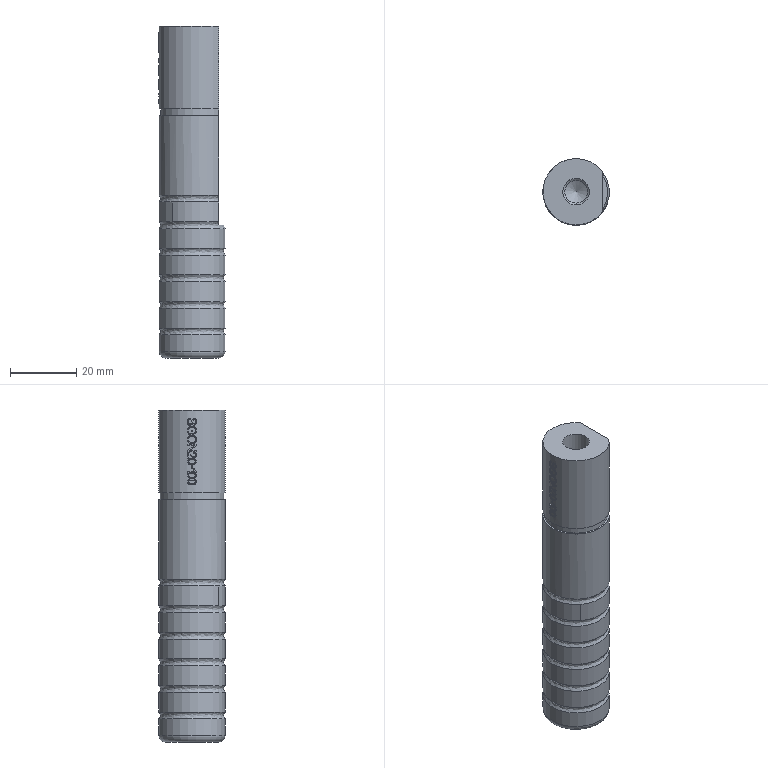Part | STEP file | PN_0060_id538_x_t | 1 solid | 178 faces | box 20 x 20 x 100 mm | volume 28952 mm3 | cylinder 85 | plane 83 | spline 7 | cone 2 | torus 1 | commonest cylinder face diameters 20 x14 19.8 x10 1.145 x3 1.367 x3 1.371 x3 1.387 x3